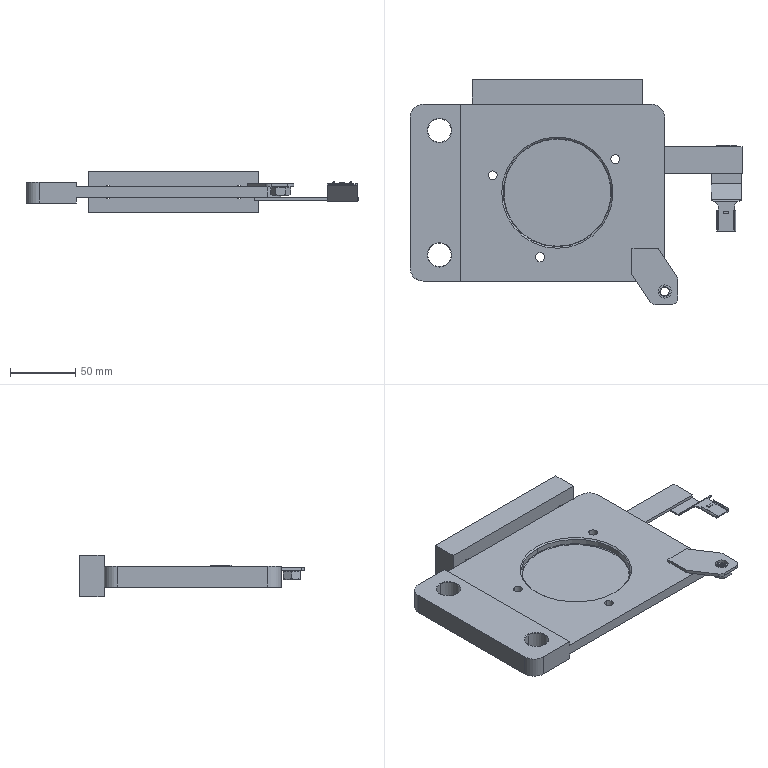Part | SolidWorks | 6 solids | 173 faces | box 253.5 x 172 x 32 mm | volume 295798 mm3 | plane 68 | cylinder 53 | cone 50 | torus 2 | commonest cylinder face diameters 6.647 x14 10 x7 6.8 x6 1 x5 3.04 x5 10.2 x4